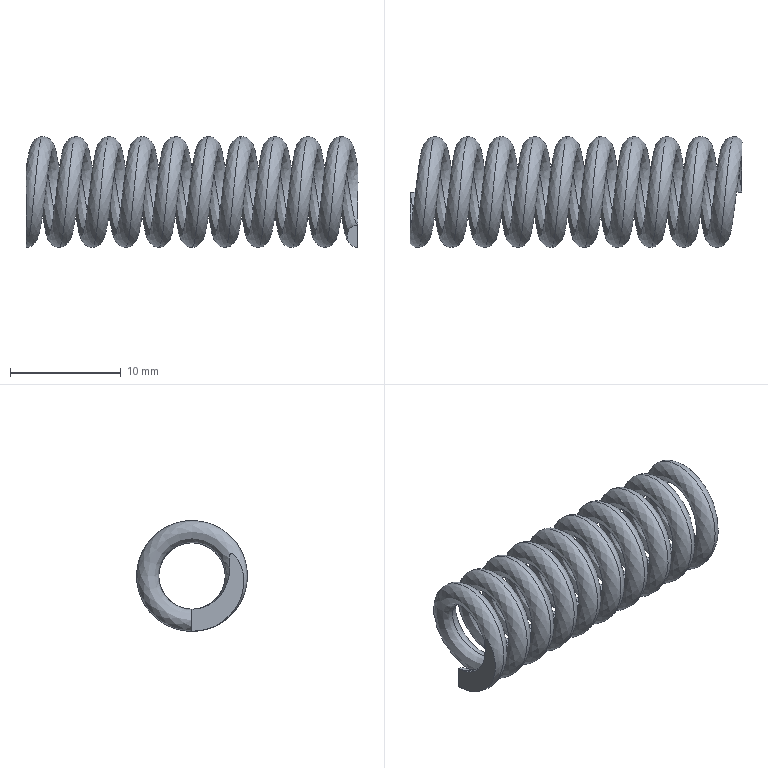Part | NX | features BREP 1 | 1 solid | 6 faces | box 30 x 10 x 10 mm | volume 778.892 mm3 | plane 4 | spline 2